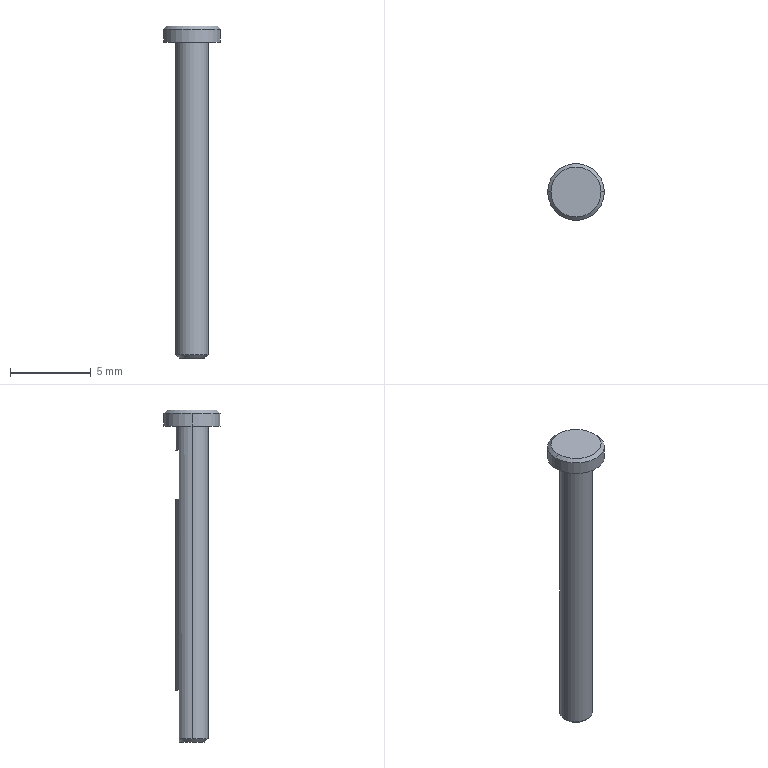Part | SolidWorks | features ICE 3, Chamfer 1, Extrusion 1 | 1 solid | 17 faces | box 3.5 x 3.5 x 20.5 mm | volume 69.56 mm3 | plane 8 | cone 5 | cylinder 4 | commonest cylinder face diameters 2 x2 3.5 x2
STEP:
#1=CARTESIAN_POINT('',(-0.8,0.,-9.75));
#2=VERTEX_POINT('',#1);
#3=CARTESIAN_POINT('',(0.,0.8,-9.75));
#4=VERTEX_POINT('',#3);
#5=CARTESIAN_POINT('',(0.,0.,-9.75));
#6=DIRECTION('',(0.,0.,-1.));
#7=DIRECTION('',(1.,0.,0.));
#8=AXIS2_PLACEMENT_3D('',#5,#6,#7);
#9=CIRCLE('',#8,0.8);
#10=EDGE_CURVE('',#2,#4,#9,.T.);
#11=ORIENTED_EDGE('',*,*,#10,.F.);
#12=CARTESIAN_POINT('',(-1.,0.,-9.55));
#13=VERTEX_POINT('',#12);
#14=CARTESIAN_POINT('',(-1.,0.,-9.55));
#15=DIRECTION('',(-0.7071,0.,0.7071));
#16=VECTOR('',#15,1000.);
#17=LINE('',#14,#16);
#18=EDGE_CURVE('',#2,#13,#17,.T.);
#19=ORIENTED_EDGE('',*,*,#18,.T.);
#20=CARTESIAN_POINT('',(-0.6,0.8,-9.55));
#21=VERTEX_POINT('',#20);
#22=CARTESIAN_POINT('',(0.,0.,-9.55));
#23=DIRECTION('',(0.,0.,1.));
#24=DIRECTION('',(1.,0.,0.));
#25=AXIS2_PLACEMENT_3D('',#22,#23,#24);
#26=CIRCLE('',#25,1.);
#27=EDGE_CURVE('',#21,#13,#26,.T.);
#28=ORIENTED_EDGE('',*,*,#27,.F.);
#29=CARTESIAN_POINT('',(0.,0.8,-9.75));
#30=CARTESIAN_POINT('',(-0.1073,0.8,-9.75));
#31=CARTESIAN_POINT('',(-0.2132,0.8,-9.727));
#32=CARTESIAN_POINT('',(-0.4127,0.8,-9.655));
#33=CARTESIAN_POINT('',(-0.5088,0.8,-9.605));
#34=CARTESIAN_POINT('',(-0.6,0.8,-9.55));
#35=B_SPLINE_CURVE_WITH_KNOTS('',3,(#29,#30,#31,#32,#33,#34),.UNSPECIFIED.,.F.,.F.,(4,2,4),(0.002974,0.003293,0.003612),.UNSPECIFIED.);
#36=EDGE_CURVE('',#4,#21,#35,.T.);
#37=ORIENTED_EDGE('',*,*,#36,.F.);
#38=EDGE_LOOP('',(#11,#19,#28,#37));
#39=FACE_OUTER_BOUND('',#38,.T.);
#40=CARTESIAN_POINT('',(0.,0.,-9.55));
#41=DIRECTION('',(0.,0.,1.));
#42=DIRECTION('',(1.,0.,0.));
#43=AXIS2_PLACEMENT_3D('',#40,#41,#42);
#44=CONICAL_SURFACE('',#43,1.,0.7854);
#45=ADVANCED_FACE('',(#39),#44,.T.);
#46=ORIENTED_EDGE('',*,*,#18,.F.);
#47=CARTESIAN_POINT('',(0.8,0.,-9.75));
#48=VERTEX_POINT('',#47);
#49=CARTESIAN_POINT('',(0.,0.,-9.75));
#50=DIRECTION('',(0.,0.,-1.));
#51=DIRECTION('',(1.,0.,0.));
#52=AXIS2_PLACEMENT_3D('',#49,#50,#51);
#53=CIRCLE('',#52,0.8);
#54=EDGE_CURVE('',#48,#2,#53,.T.);
#55=ORIENTED_EDGE('',*,*,#54,.F.);
#56=CARTESIAN_POINT('',(1.,0.,-9.55));
#57=VERTEX_POINT('',#56);
#58=CARTESIAN_POINT('',(1.,0.,-9.55));
#59=DIRECTION('',(0.7071,0.,0.7071));
#60=VECTOR('',#59,1000.);
#61=LINE('',#58,#60);
#62=EDGE_CURVE('',#48,#57,#61,.T.);
#63=ORIENTED_EDGE('',*,*,#62,.T.);
#64=CARTESIAN_POINT('',(0.,0.,-9.55));
#65=DIRECTION('',(0.,0.,1.));
#66=DIRECTION('',(1.,0.,0.));
#67=AXIS2_PLACEMENT_3D('',#64,#65,#66);
#68=CIRCLE('',#67,1.);
#69=EDGE_CURVE('',#13,#57,#68,.T.);
#70=ORIENTED_EDGE('',*,*,#69,.F.);
#71=EDGE_LOOP('',(#46,#55,#63,#70));
#72=FACE_OUTER_BOUND('',#71,.T.);
#73=CARTESIAN_POINT('',(0.,0.,-9.55));
#74=DIRECTION('',(0.,0.,1.));
#75=DIRECTION('',(1.,0.,0.));
#76=AXIS2_PLACEMENT_3D('',#73,#74,#75);
#77=CONICAL_SURFACE('',#76,1.,0.7854);
#78=ADVANCED_FACE('',(#72),#77,.T.);
#79=CARTESIAN_POINT('',(1.55,0.,10.75));
#80=VERTEX_POINT('',#79);
#81=CARTESIAN_POINT('',(-1.55,0.,10.75));
#82=VERTEX_POINT('',#81);
#83=CARTESIAN_POINT('',(0.,0.,10.75));
#84=DIRECTION('',(0.,0.,1.));
#85=DIRECTION('',(1.,0.,0.));
#86=AXIS2_PLACEMENT_3D('',#83,#84,#85);
#87=CIRCLE('',#86,1.55);
#88=EDGE_CURVE('',#80,#82,#87,.T.);
#89=ORIENTED_EDGE('',*,*,#88,.F.);
#90=CARTESIAN_POINT('',(1.75,0.,10.55));
#91=VERTEX_POINT('',#90);
#92=CARTESIAN_POINT('',(1.55,0.,10.75));
#93=DIRECTION('',(0.7071,0.,-0.7071));
#94=VECTOR('',#93,1000.);
#95=LINE('',#92,#94);
#96=EDGE_CURVE('',#80,#91,#95,.T.);
#97=ORIENTED_EDGE('',*,*,#96,.T.);
#98=CARTESIAN_POINT('',(-1.75,0.,10.55));
#99=VERTEX_POINT('',#98);
#100=CARTESIAN_POINT('',(0.,0.,10.55));
#101=DIRECTION('',(0.,0.,-1.));
#102=DIRECTION('',(1.,0.,0.));
#103=AXIS2_PLACEMENT_3D('',#100,#101,#102);
#104=CIRCLE('',#103,1.75);
#105=EDGE_CURVE('',#99,#91,#104,.T.);
#106=ORIENTED_EDGE('',*,*,#105,.F.);
#107=CARTESIAN_POINT('',(-1.55,0.,10.75));
#108=DIRECTION('',(-0.7071,0.,-0.7071));
#109=VECTOR('',#108,1000.);
#110=LINE('',#107,#109);
#111=EDGE_CURVE('',#82,#99,#110,.T.);
#112=ORIENTED_EDGE('',*,*,#111,.F.);
#113=EDGE_LOOP('',(#89,#97,#106,#112));
#114=FACE_OUTER_BOUND('',#113,.T.);
#115=CARTESIAN_POINT('',(0.,0.,10.75));
#116=DIRECTION('',(0.,0.,-1.));
#117=DIRECTION('',(-1.,0.,0.));
#118=AXIS2_PLACEMENT_3D('',#115,#116,#117);
#119=CONICAL_SURFACE('',#118,1.55,0.7854);
#120=ADVANCED_FACE('',(#114),#119,.T.);
#121=ORIENTED_EDGE('',*,*,#105,.T.);
#122=CARTESIAN_POINT('',(1.75,0.,9.75));
#123=VERTEX_POINT('',#122);
#124=CARTESIAN_POINT('',(1.75,0.,10.75));
#125=DIRECTION('',(0.,0.,-1.));
#126=VECTOR('',#125,1000.);
#127=LINE('',#124,#126);
#128=EDGE_CURVE('',#91,#123,#127,.T.);
#129=ORIENTED_EDGE('',*,*,#128,.T.);
#130=CARTESIAN_POINT('',(-1.75,0.,9.75));
#131=VERTEX_POINT('',#130);
#132=CARTESIAN_POINT('',(0.,0.,9.75));
#133=DIRECTION('',(0.,0.,1.));
#134=DIRECTION('',(1.,0.,0.));
#135=AXIS2_PLACEMENT_3D('',#132,#133,#134);
#136=CIRCLE('',#135,1.75);
#137=EDGE_CURVE('',#123,#131,#136,.T.);
#138=ORIENTED_EDGE('',*,*,#137,.T.);
#139=CARTESIAN_POINT('',(-1.75,0.,10.75));
#140=DIRECTION('',(0.,0.,-1.));
#141=VECTOR('',#140,1000.);
#142=LINE('',#139,#141);
#143=EDGE_CURVE('',#99,#131,#142,.T.);
#144=ORIENTED_EDGE('',*,*,#143,.F.);
#145=EDGE_LOOP('',(#121,#129,#138,#144));
#146=FACE_OUTER_BOUND('',#145,.T.);
#147=CARTESIAN_POINT('',(0.,0.,10.75));
#148=DIRECTION('',(0.,0.,-1.));
#149=DIRECTION('',(-1.,0.,0.));
#150=AXIS2_PLACEMENT_3D('',#147,#148,#149);
#151=CYLINDRICAL_SURFACE('',#150,1.75);
#152=ADVANCED_FACE('',(#146),#151,.T.);
#153=CARTESIAN_POINT('',(-0.6,0.8,8.25));
#154=VERTEX_POINT('',#153);
#155=CARTESIAN_POINT('',(0.6,0.8,8.25));
#156=VERTEX_POINT('',#155);
#157=CARTESIAN_POINT('',(0.,0.,8.25));
#158=DIRECTION('',(0.,0.,-1.));
#159=DIRECTION('',(-1.,0.,0.));
#160=AXIS2_PLACEMENT_3D('',#157,#158,#159);
#161=CIRCLE('',#160,1.);
#162=EDGE_CURVE('',#154,#156,#161,.T.);
#163=ORIENTED_EDGE('',*,*,#162,.F.);
#164=CARTESIAN_POINT('',(-0.6,0.8,5.25));
#165=VERTEX_POINT('',#164);
#166=CARTESIAN_POINT('',(-0.6,0.8,8.25));
#167=DIRECTION('',(0.,0.,-1.));
#168=VECTOR('',#167,1000.);
#169=LINE('',#166,#168);
#170=EDGE_CURVE('',#154,#165,#169,.T.);
#171=ORIENTED_EDGE('',*,*,#170,.T.);
#172=CARTESIAN_POINT('',(0.6,0.8,5.25));
#173=VERTEX_POINT('',#172);
#174=CARTESIAN_POINT('',(0.,0.,5.25));
#175=DIRECTION('',(0.,0.,-1.));
#176=DIRECTION('',(-1.,0.,0.));
#177=AXIS2_PLACEMENT_3D('',#174,#175,#176);
#178=CIRCLE('',#177,1.);
#179=EDGE_CURVE('',#165,#173,#178,.T.);
#180=ORIENTED_EDGE('',*,*,#179,.T.);
#181=CARTESIAN_POINT('',(0.6,0.8,8.25));
#182=DIRECTION('',(0.,0.,-1.));
#183=VECTOR('',#182,1000.);
#184=LINE('',#181,#183);
#185=EDGE_CURVE('',#156,#173,#184,.T.);
#186=ORIENTED_EDGE('',*,*,#185,.F.);
#187=EDGE_LOOP('',(#163,#171,#180,#186));
#188=FACE_BOUND('',#187,.T.);
#189=CARTESIAN_POINT('',(1.,0.,9.75));
#190=VERTEX_POINT('',#189);
#191=CARTESIAN_POINT('',(-1.,0.,9.75));
#192=VERTEX_POINT('',#191);
#193=CARTESIAN_POINT('',(0.,0.,9.75));
#194=DIRECTION('',(0.,0.,1.));
#195=DIRECTION('',(1.,0.,0.));
#196=AXIS2_PLACEMENT_3D('',#193,#194,#195);
#197=CIRCLE('',#196,1.);
#198=EDGE_CURVE('',#190,#192,#197,.T.);
#199=ORIENTED_EDGE('',*,*,#198,.F.);
#200=CARTESIAN_POINT('',(1.,0.,9.75));
#201=DIRECTION('',(0.,0.,-1.));
#202=VECTOR('',#201,1000.);
#203=LINE('',#200,#202);
#204=EDGE_CURVE('',#190,#57,#203,.T.);
#205=ORIENTED_EDGE('',*,*,#204,.T.);
#206=CARTESIAN_POINT('',(0.6,0.8,-9.55));
#207=VERTEX_POINT('',#206);
#208=CARTESIAN_POINT('',(0.,0.,-9.55));
#209=DIRECTION('',(0.,0.,1.));
#210=DIRECTION('',(1.,0.,0.));
#211=AXIS2_PLACEMENT_3D('',#208,#209,#210);
#212=CIRCLE('',#211,1.);
#213=EDGE_CURVE('',#57,#207,#212,.T.);
#214=ORIENTED_EDGE('',*,*,#213,.T.);
#215=CARTESIAN_POINT('',(0.6,0.8,-6.55));
#216=VERTEX_POINT('',#215);
#217=CARTESIAN_POINT('',(0.6,0.8,-6.55));
#218=DIRECTION('',(0.,0.,-1.));
#219=VECTOR('',#218,1000.);
#220=LINE('',#217,#219);
#221=EDGE_CURVE('',#216,#207,#220,.T.);
#222=ORIENTED_EDGE('',*,*,#221,.F.);
#223=CARTESIAN_POINT('',(-0.6,0.8,-6.55));
#224=VERTEX_POINT('',#223);
#225=CARTESIAN_POINT('',(0.,0.,-6.55));
#226=DIRECTION('',(0.,0.,-1.));
#227=DIRECTION('',(-1.,0.,0.));
#228=AXIS2_PLACEMENT_3D('',#225,#226,#227);
#229=CIRCLE('',#228,1.);
#230=EDGE_CURVE('',#224,#216,#229,.T.);
#231=ORIENTED_EDGE('',*,*,#230,.F.);
#232=CARTESIAN_POINT('',(-0.6,0.8,-6.55));
#233=DIRECTION('',(0.,0.,-1.));
#234=VECTOR('',#233,1000.);
#235=LINE('',#232,#234);
#236=EDGE_CURVE('',#224,#21,#235,.T.);
#237=ORIENTED_EDGE('',*,*,#236,.T.);
#238=ORIENTED_EDGE('',*,*,#27,.T.);
#239=CARTESIAN_POINT('',(-1.,0.,9.75));
#240=DIRECTION('',(0.,0.,-1.));
#241=VECTOR('',#240,1000.);
#242=LINE('',#239,#241);
#243=EDGE_CURVE('',#192,#13,#242,.T.);
#244=ORIENTED_EDGE('',*,*,#243,.F.);
#245=EDGE_LOOP('',(#199,#205,#214,#222,#231,#237,#238,#244));
#246=FACE_OUTER_BOUND('',#245,.T.);
#247=CARTESIAN_POINT('',(0.,0.,9.75));
#248=DIRECTION('',(0.,0.,-1.));
#249=DIRECTION('',(-1.,0.,0.));
#250=AXIS2_PLACEMENT_3D('',#247,#248,#249);
#251=CYLINDRICAL_SURFACE('',#250,1.);
#252=ADVANCED_FACE('',(#188,#246),#251,.T.);
#253=ORIENTED_EDGE('',*,*,#204,.F.);
#254=CARTESIAN_POINT('',(0.,0.,9.75));
#255=DIRECTION('',(0.,0.,1.));
#256=DIRECTION('',(1.,0.,0.));
#257=AXIS2_PLACEMENT_3D('',#254,#255,#256);
#258=CIRCLE('',#257,1.);
#259=EDGE_CURVE('',#192,#190,#258,.T.);
#260=ORIENTED_EDGE('',*,*,#259,.F.);
#261=ORIENTED_EDGE('',*,*,#243,.T.);
#262=ORIENTED_EDGE('',*,*,#69,.T.);
#263=EDGE_LOOP('',(#253,#260,#261,#262));
#264=FACE_OUTER_BOUND('',#263,.T.);
#265=CARTESIAN_POINT('',(0.,0.,9.75));
#266=DIRECTION('',(0.,0.,-1.));
#267=DIRECTION('',(-1.,0.,0.));
#268=AXIS2_PLACEMENT_3D('',#265,#266,#267);
#269=CYLINDRICAL_SURFACE('',#268,1.);
#270=ADVANCED_FACE('',(#264),#269,.T.);
#271=CARTESIAN_POINT('',(0.,0.,-9.75));
#272=DIRECTION('',(0.,0.,-1.));
#273=DIRECTION('',(1.,0.,0.));
#274=AXIS2_PLACEMENT_3D('',#271,#272,#273);
#275=CIRCLE('',#274,0.8);
#276=EDGE_CURVE('',#4,#48,#275,.T.);
#277=ORIENTED_EDGE('',*,*,#276,.T.);
#278=ORIENTED_EDGE('',*,*,#54,.T.);
#279=ORIENTED_EDGE('',*,*,#10,.T.);
#280=EDGE_LOOP('',(#277,#278,#279));
#281=FACE_OUTER_BOUND('',#280,.T.);
#282=CARTESIAN_POINT('',(0.,0.,-9.75));
#283=DIRECTION('',(0.,0.,1.));
#284=DIRECTION('',(1.,0.,0.));
#285=AXIS2_PLACEMENT_3D('',#282,#283,#284);
#286=PLANE('',#285);
#287=ADVANCED_FACE('',(#281),#286,.F.);
#288=CARTESIAN_POINT('',(0.,0.,9.75));
#289=DIRECTION('',(0.,0.,1.));
#290=DIRECTION('',(1.,0.,0.));
#291=AXIS2_PLACEMENT_3D('',#288,#289,#290);
#292=CIRCLE('',#291,1.75);
#293=EDGE_CURVE('',#131,#123,#292,.T.);
#294=ORIENTED_EDGE('',*,*,#293,.F.);
#295=ORIENTED_EDGE('',*,*,#137,.F.);
#296=EDGE_LOOP('',(#294,#295));
#297=FACE_OUTER_BOUND('',#296,.T.);
#298=ORIENTED_EDGE('',*,*,#259,.T.);
#299=ORIENTED_EDGE('',*,*,#198,.T.);
#300=EDGE_LOOP('',(#298,#299));
#301=FACE_BOUND('',#300,.T.);
#302=CARTESIAN_POINT('',(0.,0.,9.75));
#303=DIRECTION('',(0.,0.,1.));
#304=DIRECTION('',(1.,0.,0.));
#305=AXIS2_PLACEMENT_3D('',#302,#303,#304);
#306=PLANE('',#305);
#307=ADVANCED_FACE('',(#297,#301),#306,.F.);
#308=ORIENTED_EDGE('',*,*,#128,.F.);
#309=CARTESIAN_POINT('',(0.,0.,10.55));
#310=DIRECTION('',(0.,0.,-1.));
#311=DIRECTION('',(1.,0.,0.));
#312=AXIS2_PLACEMENT_3D('',#309,#310,#311);
#313=CIRCLE('',#312,1.75);
#314=EDGE_CURVE('',#91,#99,#313,.T.);
#315=ORIENTED_EDGE('',*,*,#314,.T.);
#316=ORIENTED_EDGE('',*,*,#143,.T.);
#317=ORIENTED_EDGE('',*,*,#293,.T.);
#318=EDGE_LOOP('',(#308,#315,#316,#317));
#319=FACE_OUTER_BOUND('',#318,.T.);
#320=CARTESIAN_POINT('',(0.,0.,10.75));
#321=DIRECTION('',(0.,0.,-1.));
#322=DIRECTION('',(-1.,0.,0.));
#323=AXIS2_PLACEMENT_3D('',#320,#321,#322);
#324=CYLINDRICAL_SURFACE('',#323,1.75);
#325=ADVANCED_FACE('',(#319),#324,.T.);
#326=CARTESIAN_POINT('',(0.,0.,10.75));
#327=DIRECTION('',(0.,0.,1.));
#328=DIRECTION('',(1.,0.,0.));
#329=AXIS2_PLACEMENT_3D('',#326,#327,#328);
#330=CIRCLE('',#329,1.55);
#331=EDGE_CURVE('',#82,#80,#330,.T.);
#332=ORIENTED_EDGE('',*,*,#331,.T.);
#333=ORIENTED_EDGE('',*,*,#88,.T.);
#334=EDGE_LOOP('',(#332,#333));
#335=FACE_OUTER_BOUND('',#334,.T.);
#336=CARTESIAN_POINT('',(0.,0.,10.75));
#337=DIRECTION('',(0.,0.,1.));
#338=DIRECTION('',(1.,0.,0.));
#339=AXIS2_PLACEMENT_3D('',#336,#337,#338);
#340=PLANE('',#339);
#341=ADVANCED_FACE('',(#335),#340,.T.);
#342=ORIENTED_EDGE('',*,*,#96,.F.);
#343=ORIENTED_EDGE('',*,*,#331,.F.);
#344=ORIENTED_EDGE('',*,*,#111,.T.);
#345=ORIENTED_EDGE('',*,*,#314,.F.);
#346=EDGE_LOOP('',(#342,#343,#344,#345));
#347=FACE_OUTER_BOUND('',#346,.T.);
#348=CARTESIAN_POINT('',(0.,0.,10.75));
#349=DIRECTION('',(0.,0.,-1.));
#350=DIRECTION('',(-1.,0.,0.));
#351=AXIS2_PLACEMENT_3D('',#348,#349,#350);
#352=CONICAL_SURFACE('',#351,1.55,0.7854);
#353=ADVANCED_FACE('',(#347),#352,.T.);
#354=ORIENTED_EDGE('',*,*,#62,.F.);
#355=ORIENTED_EDGE('',*,*,#276,.F.);
#356=CARTESIAN_POINT('',(0.6,0.8,-9.55));
#357=CARTESIAN_POINT('',(0.5084,0.8,-9.605));
#358=CARTESIAN_POINT('',(0.414,0.8,-9.654));
#359=CARTESIAN_POINT('',(0.2131,0.8,-9.727));
#360=CARTESIAN_POINT('',(0.1071,0.8,-9.75));
#361=CARTESIAN_POINT('',(0.,0.8,-9.75));
#362=B_SPLINE_CURVE_WITH_KNOTS('',3,(#356,#357,#358,#359,#360,#361),.UNSPECIFIED.,.F.,.F.,(4,2,4),(0.002338,0.002656,0.002974),.UNSPECIFIED.);
#363=EDGE_CURVE('',#207,#4,#362,.T.);
#364=ORIENTED_EDGE('',*,*,#363,.F.);
#365=ORIENTED_EDGE('',*,*,#213,.F.);
#366=EDGE_LOOP('',(#354,#355,#364,#365));
#367=FACE_OUTER_BOUND('',#366,.T.);
#368=CARTESIAN_POINT('',(0.,0.,-9.55));
#369=DIRECTION('',(0.,0.,1.));
#370=DIRECTION('',(1.,0.,0.));
#371=AXIS2_PLACEMENT_3D('',#368,#369,#370);
#372=CONICAL_SURFACE('',#371,1.,0.7854);
#373=ADVANCED_FACE('',(#367),#372,.T.);
#374=ORIENTED_EDGE('',*,*,#363,.T.);
#375=ORIENTED_EDGE('',*,*,#36,.T.);
#376=ORIENTED_EDGE('',*,*,#236,.F.);
#377=CARTESIAN_POINT('',(0.6,0.8,-6.55));
#378=DIRECTION('',(-1.,0.,0.));
#379=VECTOR('',#378,1000.);
#380=LINE('',#377,#379);
#381=EDGE_CURVE('',#216,#224,#380,.T.);
#382=ORIENTED_EDGE('',*,*,#381,.F.);
#383=ORIENTED_EDGE('',*,*,#221,.T.);
#384=EDGE_LOOP('',(#374,#375,#376,#382,#383));
#385=FACE_OUTER_BOUND('',#384,.T.);
#386=CARTESIAN_POINT('',(0.6,0.8,-6.55));
#387=DIRECTION('',(0.,-1.,0.));
#388=DIRECTION('',(0.,0.,-1.));
#389=AXIS2_PLACEMENT_3D('',#386,#387,#388);
#390=PLANE('',#389);
#391=ADVANCED_FACE('',(#385),#390,.F.);
#392=ORIENTED_EDGE('',*,*,#230,.T.);
#393=ORIENTED_EDGE('',*,*,#381,.T.);
#394=EDGE_LOOP('',(#392,#393));
#395=FACE_OUTER_BOUND('',#394,.T.);
#396=CARTESIAN_POINT('',(0.,0.,-6.55));
#397=DIRECTION('',(0.,0.,-1.));
#398=DIRECTION('',(-1.,0.,0.));
#399=AXIS2_PLACEMENT_3D('',#396,#397,#398);
#400=PLANE('',#399);
#401=ADVANCED_FACE('',(#395),#400,.T.);
#402=CARTESIAN_POINT('',(0.6,0.8,5.25));
#403=DIRECTION('',(-1.,0.,0.));
#404=VECTOR('',#403,1000.);
#405=LINE('',#402,#404);
#406=EDGE_CURVE('',#173,#165,#405,.T.);
#407=ORIENTED_EDGE('',*,*,#406,.T.);
#408=ORIENTED_EDGE('',*,*,#170,.F.);
#409=CARTESIAN_POINT('',(0.6,0.8,8.25));
#410=DIRECTION('',(-1.,0.,0.));
#411=VECTOR('',#410,1000.);
#412=LINE('',#409,#411);
#413=EDGE_CURVE('',#156,#154,#412,.T.);
#414=ORIENTED_EDGE('',*,*,#413,.F.);
#415=ORIENTED_EDGE('',*,*,#185,.T.);
#416=EDGE_LOOP('',(#407,#408,#414,#415));
#417=FACE_OUTER_BOUND('',#416,.T.);
#418=CARTESIAN_POINT('',(0.6,0.8,8.25));
#419=DIRECTION('',(0.,-1.,0.));
#420=DIRECTION('',(0.,0.,-1.));
#421=AXIS2_PLACEMENT_3D('',#418,#419,#420);
#422=PLANE('',#421);
#423=ADVANCED_FACE('',(#417),#422,.F.);
#424=ORIENTED_EDGE('',*,*,#162,.T.);
#425=ORIENTED_EDGE('',*,*,#413,.T.);
#426=EDGE_LOOP('',(#424,#425));
#427=FACE_OUTER_BOUND('',#426,.T.);
#428=CARTESIAN_POINT('',(0.,0.,8.25));
#429=DIRECTION('',(0.,0.,-1.));
#430=DIRECTION('',(-1.,0.,0.));
#431=AXIS2_PLACEMENT_3D('',#428,#429,#430);
#432=PLANE('',#431);
#433=ADVANCED_FACE('',(#427),#432,.T.);
#434=ORIENTED_EDGE('',*,*,#179,.F.);
#435=ORIENTED_EDGE('',*,*,#406,.F.);
#436=EDGE_LOOP('',(#434,#435));
#437=FACE_OUTER_BOUND('',#436,.T.);
#438=CARTESIAN_POINT('',(0.,0.,5.25));
#439=DIRECTION('',(0.,0.,-1.));
#440=DIRECTION('',(-1.,0.,0.));
#441=AXIS2_PLACEMENT_3D('',#438,#439,#440);
#442=PLANE('',#441);
#443=ADVANCED_FACE('',(#437),#442,.F.);
#444=CLOSED_SHELL('',(#45,#78,#120,#152,#252,#270,#287,#307,#325,#341,#353,#373,#391,#401,#423,#433,#443));
#445=MANIFOLD_SOLID_BREP('',#444);
#446=CARTESIAN_POINT('',(0.,0.,0.));
#447=DIRECTION('',(0.,0.,1.));
#448=DIRECTION('',(1.,0.,0.));
#449=AXIS2_PLACEMENT_3D('',#446,#447,#448);
#450=(LENGTH_UNIT()NAMED_UNIT(*)SI_UNIT(.MILLI.,.METRE.));
#451=UNCERTAINTY_MEASURE_WITH_UNIT(LENGTH_MEASURE(0.00001),#450,'','');
#452=(NAMED_UNIT(*)PLANE_ANGLE_UNIT()SI_UNIT($,.RADIAN.));
#453=(NAMED_UNIT(*)SI_UNIT($,.STERADIAN.)SOLID_ANGLE_UNIT());
#454=(GEOMETRIC_REPRESENTATION_CONTEXT(3)GLOBAL_UNCERTAINTY_ASSIGNED_CONTEXT((#451))GLOBAL_UNIT_ASSIGNED_CONTEXT((#450,#452,#453))REPRESENTATION_CONTEXT('',''));
#455=ADVANCED_BREP_SHAPE_REPRESENTATION('',(#445,#449),#454);